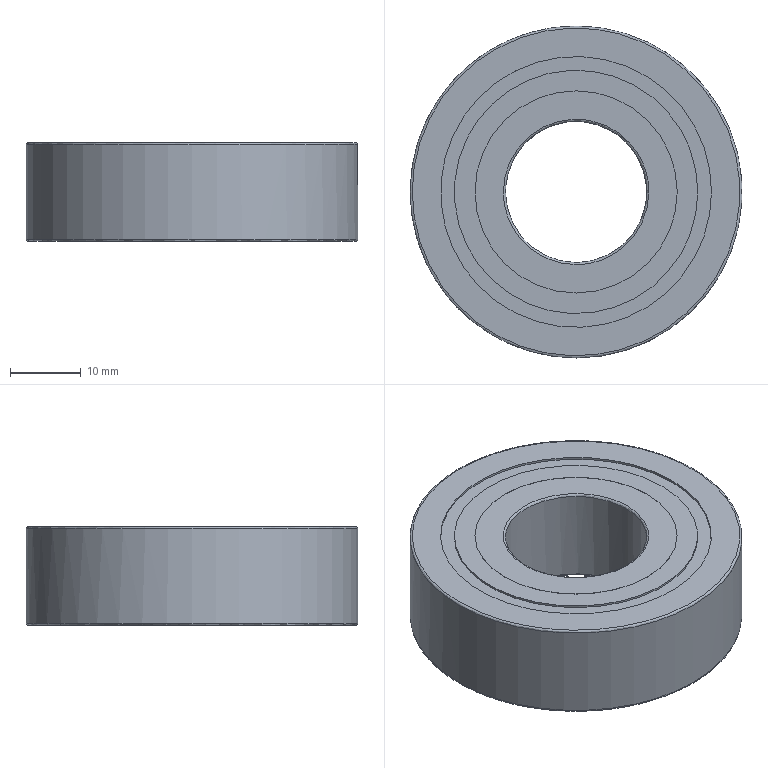Part | NX | 1 solid | 20 faces | box 47 x 47 x 14 mm | volume 19738 mm3 | cylinder 8 | spline 6 | plane 6 | commonest cylinder face diameters 28.64 x2 34.46 x2 38.36 x2 20 x1 47 x1